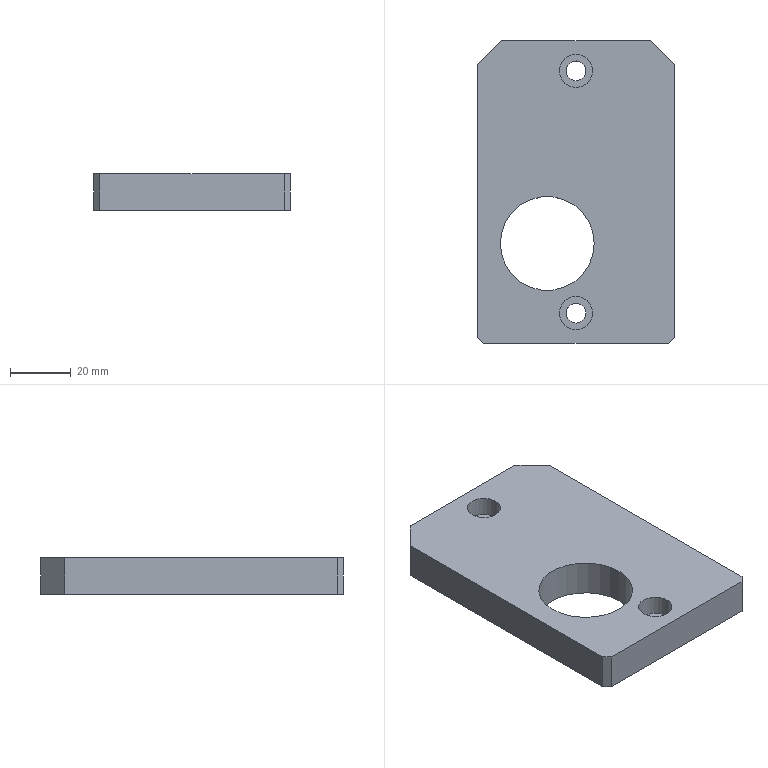Part | STEP file | P011002NM05-000 | 1 solid | 17 faces | box 65 x 100 x 12 mm | volume 66526 mm3 | plane 12 | cylinder 5 | commonest cylinder face diameters 6.5 x2 11 x2 31 x1
STEP:
#1=CARTESIAN_POINT('',(0.,0.,0.));
#2=DIRECTION('',(0.,0.,1.));
#3=DIRECTION('',(1.,0.,0.));
#4=AXIS2_PLACEMENT_3D('',#1,#2,#3);
#5=CARTESIAN_POINT('',(178.,-325.,9.));
#6=VERTEX_POINT('',#5);
#7=CARTESIAN_POINT('',(117.,-325.,9.));
#8=VERTEX_POINT('',#7);
#9=CARTESIAN_POINT('',(-325.,-325.,9.));
#10=DIRECTION('',(-1.,0.,0.));
#11=VECTOR('',#10,1.);
#12=LINE('',#9,#11);
#13=CARTESIAN_POINT('',(-325.,-325.,260.));
#14=DIRECTION('',(0.,1.,0.));
#15=DIRECTION('',(0.,0.,1.));
#16=AXIS2_PLACEMENT_3D('',#13,#14,#15);
#17=PLANE('',#16);
#18=CARTESIAN_POINT('',(-251.,0.));
#19=DIRECTION('',(0.,-1.));
#20=VECTOR('',#19,1.);
#21=LINE('',#18,#20);
#22=(GEOMETRIC_REPRESENTATION_CONTEXT(2)PARAMETRIC_REPRESENTATION_CONTEXT()REPRESENTATION_CONTEXT('',''));
#23=DEFINITIONAL_REPRESENTATION('',(#21),#22);
#24=PCURVE('',#17,#23);
#25=CARTESIAN_POINT('',(178.,-325.,9.));
#26=DIRECTION('',(0.,0.,1.));
#27=DIRECTION('',(1.,0.,0.));
#28=AXIS2_PLACEMENT_3D('',#25,#26,#27);
#29=PLANE('',#28);
#30=CARTESIAN_POINT('',(-503.,0.));
#31=DIRECTION('',(-1.,0.));
#32=VECTOR('',#31,1.);
#33=LINE('',#30,#32);
#34=(GEOMETRIC_REPRESENTATION_CONTEXT(2)PARAMETRIC_REPRESENTATION_CONTEXT()REPRESENTATION_CONTEXT('',''));
#35=DEFINITIONAL_REPRESENTATION('',(#33),#34);
#36=PCURVE('',#29,#35);
#37=SURFACE_CURVE('',#12,(#24,#36),.PCURVE_S1.);
#38=EDGE_CURVE('',#6,#8,#37,.T.);
#39=ORIENTED_EDGE('',*,*,#38,.F.);
#40=CARTESIAN_POINT('',(178.,-325.,21.));
#41=VERTEX_POINT('',#40);
#42=CARTESIAN_POINT('',(178.,-325.,260.));
#43=DIRECTION('',(0.,0.,1.));
#44=VECTOR('',#43,1.);
#45=LINE('',#42,#44);
#46=CARTESIAN_POINT('',(0.,503.));
#47=DIRECTION('',(1.,0.));
#48=VECTOR('',#47,1.);
#49=LINE('',#46,#48);
#50=(GEOMETRIC_REPRESENTATION_CONTEXT(2)PARAMETRIC_REPRESENTATION_CONTEXT()REPRESENTATION_CONTEXT('',''));
#51=DEFINITIONAL_REPRESENTATION('',(#49),#50);
#52=PCURVE('',#17,#51);
#53=CARTESIAN_POINT('',(180.,-323.,21.));
#54=DIRECTION('',(-0.7071,0.7071,0.));
#55=DIRECTION('',(-0.7071,-0.7071,0.));
#56=AXIS2_PLACEMENT_3D('',#53,#54,#55);
#57=PLANE('',#56);
#58=CARTESIAN_POINT('',(2.828,239.));
#59=DIRECTION('',(0.,1.));
#60=VECTOR('',#59,1.);
#61=LINE('',#58,#60);
#62=(GEOMETRIC_REPRESENTATION_CONTEXT(2)PARAMETRIC_REPRESENTATION_CONTEXT()REPRESENTATION_CONTEXT('',''));
#63=DEFINITIONAL_REPRESENTATION('',(#61),#62);
#64=PCURVE('',#57,#63);
#65=SURFACE_CURVE('',#45,(#52,#64),.PCURVE_S1.);
#66=EDGE_CURVE('',#6,#41,#65,.T.);
#67=ORIENTED_EDGE('',*,*,#66,.T.);
#68=CARTESIAN_POINT('',(117.,-325.,21.));
#69=VERTEX_POINT('',#68);
#70=CARTESIAN_POINT('',(-325.,-325.,21.));
#71=DIRECTION('',(-1.,0.,0.));
#72=VECTOR('',#71,1.);
#73=LINE('',#70,#72);
#74=CARTESIAN_POINT('',(-239.,0.));
#75=DIRECTION('',(0.,-1.));
#76=VECTOR('',#75,1.);
#77=LINE('',#74,#76);
#78=(GEOMETRIC_REPRESENTATION_CONTEXT(2)PARAMETRIC_REPRESENTATION_CONTEXT()REPRESENTATION_CONTEXT('',''));
#79=DEFINITIONAL_REPRESENTATION('',(#77),#78);
#80=PCURVE('',#17,#79);
#81=CARTESIAN_POINT('',(150.,-240.,21.));
#82=DIRECTION('',(0.,0.,1.));
#83=DIRECTION('',(1.,0.,0.));
#84=AXIS2_PLACEMENT_3D('',#81,#82,#83);
#85=PLANE('',#84);
#86=CARTESIAN_POINT('',(-475.,-85.));
#87=DIRECTION('',(-1.,0.));
#88=VECTOR('',#87,1.);
#89=LINE('',#86,#88);
#90=(GEOMETRIC_REPRESENTATION_CONTEXT(2)PARAMETRIC_REPRESENTATION_CONTEXT()REPRESENTATION_CONTEXT('',''));
#91=DEFINITIONAL_REPRESENTATION('',(#89),#90);
#92=PCURVE('',#85,#91);
#93=SURFACE_CURVE('',#73,(#80,#92),.PCURVE_S1.);
#94=EDGE_CURVE('',#41,#69,#93,.T.);
#95=ORIENTED_EDGE('',*,*,#94,.T.);
#96=CARTESIAN_POINT('',(117.,-325.,260.));
#97=DIRECTION('',(0.,0.,-1.));
#98=VECTOR('',#97,1.);
#99=LINE('',#96,#98);
#100=CARTESIAN_POINT('',(0.,442.));
#101=DIRECTION('',(-1.,0.));
#102=VECTOR('',#101,1.);
#103=LINE('',#100,#102);
#104=(GEOMETRIC_REPRESENTATION_CONTEXT(2)PARAMETRIC_REPRESENTATION_CONTEXT()REPRESENTATION_CONTEXT('',''));
#105=DEFINITIONAL_REPRESENTATION('',(#103),#104);
#106=PCURVE('',#17,#105);
#107=CARTESIAN_POINT('',(117.,-325.,260.));
#108=DIRECTION('',(0.7071,0.7071,0.));
#109=DIRECTION('',(-0.7071,0.7071,0.));
#110=AXIS2_PLACEMENT_3D('',#107,#108,#109);
#111=PLANE('',#110);
#112=CARTESIAN_POINT('',(0.,0.));
#113=DIRECTION('',(0.,-1.));
#114=VECTOR('',#113,1.);
#115=LINE('',#112,#114);
#116=(GEOMETRIC_REPRESENTATION_CONTEXT(2)PARAMETRIC_REPRESENTATION_CONTEXT()REPRESENTATION_CONTEXT('',''));
#117=DEFINITIONAL_REPRESENTATION('',(#115),#116);
#118=PCURVE('',#111,#117);
#119=SURFACE_CURVE('',#99,(#106,#118),.PCURVE_S1.);
#120=EDGE_CURVE('',#69,#8,#119,.T.);
#121=ORIENTED_EDGE('',*,*,#120,.T.);
#122=EDGE_LOOP('',(#39,#67,#95,#121));
#123=FACE_BOUND('',#122,.T.);
#124=ADVANCED_FACE('',(#123),#17,.F.);
#125=CARTESIAN_POINT('',(180.,-233.,9.));
#126=VERTEX_POINT('',#125);
#127=CARTESIAN_POINT('',(180.,-323.,9.));
#128=VERTEX_POINT('',#127);
#129=CARTESIAN_POINT('',(180.,-225.,9.));
#130=DIRECTION('',(0.,-1.,0.));
#131=VECTOR('',#130,1.);
#132=LINE('',#129,#131);
#133=CARTESIAN_POINT('',(180.,-225.,21.));
#134=DIRECTION('',(-1.,0.,0.));
#135=DIRECTION('',(0.,0.,-1.));
#136=AXIS2_PLACEMENT_3D('',#133,#134,#135);
#137=PLANE('',#136);
#138=CARTESIAN_POINT('',(12.,0.));
#139=DIRECTION('',(0.,1.));
#140=VECTOR('',#139,1.);
#141=LINE('',#138,#140);
#142=(GEOMETRIC_REPRESENTATION_CONTEXT(2)PARAMETRIC_REPRESENTATION_CONTEXT()REPRESENTATION_CONTEXT('',''));
#143=DEFINITIONAL_REPRESENTATION('',(#141),#142);
#144=PCURVE('',#137,#143);
#145=CARTESIAN_POINT('',(2.,100.));
#146=DIRECTION('',(0.,-1.));
#147=VECTOR('',#146,1.);
#148=LINE('',#145,#147);
#149=(GEOMETRIC_REPRESENTATION_CONTEXT(2)PARAMETRIC_REPRESENTATION_CONTEXT()REPRESENTATION_CONTEXT('',''));
#150=DEFINITIONAL_REPRESENTATION('',(#148),#149);
#151=PCURVE('',#29,#150);
#152=SURFACE_CURVE('',#132,(#144,#151),.PCURVE_S1.);
#153=EDGE_CURVE('',#126,#128,#152,.T.);
#154=ORIENTED_EDGE('',*,*,#153,.F.);
#155=CARTESIAN_POINT('',(180.,-233.,21.));
#156=VERTEX_POINT('',#155);
#157=CARTESIAN_POINT('',(180.,-233.,21.));
#158=DIRECTION('',(0.,0.,1.));
#159=VECTOR('',#158,1.);
#160=LINE('',#157,#159);
#161=CARTESIAN_POINT('',(0.,8.));
#162=DIRECTION('',(-1.,0.));
#163=VECTOR('',#162,1.);
#164=LINE('',#161,#163);
#165=(GEOMETRIC_REPRESENTATION_CONTEXT(2)PARAMETRIC_REPRESENTATION_CONTEXT()REPRESENTATION_CONTEXT('',''));
#166=DEFINITIONAL_REPRESENTATION('',(#164),#165);
#167=PCURVE('',#137,#166);
#168=CARTESIAN_POINT('',(172.,-225.,21.));
#169=DIRECTION('',(-0.7071,-0.7071,0.));
#170=DIRECTION('',(0.7071,-0.7071,0.));
#171=AXIS2_PLACEMENT_3D('',#168,#169,#170);
#172=PLANE('',#171);
#173=CARTESIAN_POINT('',(11.314,0.));
#174=DIRECTION('',(0.,1.));
#175=VECTOR('',#174,1.);
#176=LINE('',#173,#175);
#177=(GEOMETRIC_REPRESENTATION_CONTEXT(2)PARAMETRIC_REPRESENTATION_CONTEXT()REPRESENTATION_CONTEXT('',''));
#178=DEFINITIONAL_REPRESENTATION('',(#176),#177);
#179=PCURVE('',#172,#178);
#180=SURFACE_CURVE('',#160,(#167,#179),.PCURVE_S1.);
#181=EDGE_CURVE('',#126,#156,#180,.T.);
#182=ORIENTED_EDGE('',*,*,#181,.T.);
#183=CARTESIAN_POINT('',(180.,-323.,21.));
#184=VERTEX_POINT('',#183);
#185=CARTESIAN_POINT('',(180.,-225.,21.));
#186=DIRECTION('',(0.,-1.,0.));
#187=VECTOR('',#186,1.);
#188=LINE('',#185,#187);
#189=CARTESIAN_POINT('',(0.,0.));
#190=DIRECTION('',(0.,1.));
#191=VECTOR('',#190,1.);
#192=LINE('',#189,#191);
#193=(GEOMETRIC_REPRESENTATION_CONTEXT(2)PARAMETRIC_REPRESENTATION_CONTEXT()REPRESENTATION_CONTEXT('',''));
#194=DEFINITIONAL_REPRESENTATION('',(#192),#193);
#195=PCURVE('',#137,#194);
#196=CARTESIAN_POINT('',(30.,15.));
#197=DIRECTION('',(0.,-1.));
#198=VECTOR('',#197,1.);
#199=LINE('',#196,#198);
#200=(GEOMETRIC_REPRESENTATION_CONTEXT(2)PARAMETRIC_REPRESENTATION_CONTEXT()REPRESENTATION_CONTEXT('',''));
#201=DEFINITIONAL_REPRESENTATION('',(#199),#200);
#202=PCURVE('',#85,#201);
#203=SURFACE_CURVE('',#188,(#195,#202),.PCURVE_S1.);
#204=EDGE_CURVE('',#156,#184,#203,.T.);
#205=ORIENTED_EDGE('',*,*,#204,.T.);
#206=CARTESIAN_POINT('',(180.,-323.,21.));
#207=DIRECTION('',(0.,0.,-1.));
#208=VECTOR('',#207,1.);
#209=LINE('',#206,#208);
#210=CARTESIAN_POINT('',(0.,98.));
#211=DIRECTION('',(1.,0.));
#212=VECTOR('',#211,1.);
#213=LINE('',#210,#212);
#214=(GEOMETRIC_REPRESENTATION_CONTEXT(2)PARAMETRIC_REPRESENTATION_CONTEXT()REPRESENTATION_CONTEXT('',''));
#215=DEFINITIONAL_REPRESENTATION('',(#213),#214);
#216=PCURVE('',#137,#215);
#217=CARTESIAN_POINT('',(0.,0.));
#218=DIRECTION('',(0.,-1.));
#219=VECTOR('',#218,1.);
#220=LINE('',#217,#219);
#221=(GEOMETRIC_REPRESENTATION_CONTEXT(2)PARAMETRIC_REPRESENTATION_CONTEXT()REPRESENTATION_CONTEXT('',''));
#222=DEFINITIONAL_REPRESENTATION('',(#220),#221);
#223=PCURVE('',#57,#222);
#224=SURFACE_CURVE('',#209,(#216,#223),.PCURVE_S1.);
#225=EDGE_CURVE('',#184,#128,#224,.T.);
#226=ORIENTED_EDGE('',*,*,#225,.T.);
#227=EDGE_LOOP('',(#154,#182,#205,#226));
#228=FACE_BOUND('',#227,.T.);
#229=ADVANCED_FACE('',(#228),#137,.F.);
#230=CARTESIAN_POINT('',(123.,-225.,9.));
#231=VERTEX_POINT('',#230);
#232=CARTESIAN_POINT('',(172.,-225.,9.));
#233=VERTEX_POINT('',#232);
#234=CARTESIAN_POINT('',(125.,-225.,9.));
#235=DIRECTION('',(1.,0.,0.));
#236=VECTOR('',#235,1.);
#237=LINE('',#234,#236);
#238=CARTESIAN_POINT('',(125.,-225.,21.));
#239=DIRECTION('',(0.,-1.,0.));
#240=DIRECTION('',(0.,0.,-1.));
#241=AXIS2_PLACEMENT_3D('',#238,#239,#240);
#242=PLANE('',#241);
#243=CARTESIAN_POINT('',(12.,0.));
#244=DIRECTION('',(0.,1.));
#245=VECTOR('',#244,1.);
#246=LINE('',#243,#245);
#247=(GEOMETRIC_REPRESENTATION_CONTEXT(2)PARAMETRIC_REPRESENTATION_CONTEXT()REPRESENTATION_CONTEXT('',''));
#248=DEFINITIONAL_REPRESENTATION('',(#246),#247);
#249=PCURVE('',#242,#248);
#250=CARTESIAN_POINT('',(-53.,100.));
#251=DIRECTION('',(1.,0.));
#252=VECTOR('',#251,1.);
#253=LINE('',#250,#252);
#254=(GEOMETRIC_REPRESENTATION_CONTEXT(2)PARAMETRIC_REPRESENTATION_CONTEXT()REPRESENTATION_CONTEXT('',''));
#255=DEFINITIONAL_REPRESENTATION('',(#253),#254);
#256=PCURVE('',#29,#255);
#257=SURFACE_CURVE('',#237,(#249,#256),.PCURVE_S1.);
#258=EDGE_CURVE('',#231,#233,#257,.T.);
#259=ORIENTED_EDGE('',*,*,#258,.F.);
#260=CARTESIAN_POINT('',(123.,-225.,21.));
#261=VERTEX_POINT('',#260);
#262=CARTESIAN_POINT('',(123.,-225.,21.));
#263=DIRECTION('',(0.,0.,1.));
#264=VECTOR('',#263,1.);
#265=LINE('',#262,#264);
#266=CARTESIAN_POINT('',(0.,-2.));
#267=DIRECTION('',(-1.,0.));
#268=VECTOR('',#267,1.);
#269=LINE('',#266,#268);
#270=(GEOMETRIC_REPRESENTATION_CONTEXT(2)PARAMETRIC_REPRESENTATION_CONTEXT()REPRESENTATION_CONTEXT('',''));
#271=DEFINITIONAL_REPRESENTATION('',(#269),#270);
#272=PCURVE('',#242,#271);
#273=CARTESIAN_POINT('',(115.,-233.,21.));
#274=DIRECTION('',(0.7071,-0.7071,0.));
#275=DIRECTION('',(0.7071,0.7071,0.));
#276=AXIS2_PLACEMENT_3D('',#273,#274,#275);
#277=PLANE('',#276);
#278=CARTESIAN_POINT('',(11.314,0.));
#279=DIRECTION('',(0.,1.));
#280=VECTOR('',#279,1.);
#281=LINE('',#278,#280);
#282=(GEOMETRIC_REPRESENTATION_CONTEXT(2)PARAMETRIC_REPRESENTATION_CONTEXT()REPRESENTATION_CONTEXT('',''));
#283=DEFINITIONAL_REPRESENTATION('',(#281),#282);
#284=PCURVE('',#277,#283);
#285=SURFACE_CURVE('',#265,(#272,#284),.PCURVE_S1.);
#286=EDGE_CURVE('',#231,#261,#285,.T.);
#287=ORIENTED_EDGE('',*,*,#286,.T.);
#288=CARTESIAN_POINT('',(172.,-225.,21.));
#289=VERTEX_POINT('',#288);
#290=CARTESIAN_POINT('',(125.,-225.,21.));
#291=DIRECTION('',(1.,0.,0.));
#292=VECTOR('',#291,1.);
#293=LINE('',#290,#292);
#294=CARTESIAN_POINT('',(0.,0.));
#295=DIRECTION('',(0.,1.));
#296=VECTOR('',#295,1.);
#297=LINE('',#294,#296);
#298=(GEOMETRIC_REPRESENTATION_CONTEXT(2)PARAMETRIC_REPRESENTATION_CONTEXT()REPRESENTATION_CONTEXT('',''));
#299=DEFINITIONAL_REPRESENTATION('',(#297),#298);
#300=PCURVE('',#242,#299);
#301=CARTESIAN_POINT('',(-25.,15.));
#302=DIRECTION('',(1.,0.));
#303=VECTOR('',#302,1.);
#304=LINE('',#301,#303);
#305=(GEOMETRIC_REPRESENTATION_CONTEXT(2)PARAMETRIC_REPRESENTATION_CONTEXT()REPRESENTATION_CONTEXT('',''));
#306=DEFINITIONAL_REPRESENTATION('',(#304),#305);
#307=PCURVE('',#85,#306);
#308=SURFACE_CURVE('',#293,(#300,#307),.PCURVE_S1.);
#309=EDGE_CURVE('',#261,#289,#308,.T.);
#310=ORIENTED_EDGE('',*,*,#309,.T.);
#311=CARTESIAN_POINT('',(172.,-225.,21.));
#312=DIRECTION('',(0.,0.,-1.));
#313=VECTOR('',#312,1.);
#314=LINE('',#311,#313);
#315=CARTESIAN_POINT('',(0.,47.));
#316=DIRECTION('',(1.,0.));
#317=VECTOR('',#316,1.);
#318=LINE('',#315,#317);
#319=(GEOMETRIC_REPRESENTATION_CONTEXT(2)PARAMETRIC_REPRESENTATION_CONTEXT()REPRESENTATION_CONTEXT('',''));
#320=DEFINITIONAL_REPRESENTATION('',(#318),#319);
#321=PCURVE('',#242,#320);
#322=CARTESIAN_POINT('',(0.,0.));
#323=DIRECTION('',(0.,-1.));
#324=VECTOR('',#323,1.);
#325=LINE('',#322,#324);
#326=(GEOMETRIC_REPRESENTATION_CONTEXT(2)PARAMETRIC_REPRESENTATION_CONTEXT()REPRESENTATION_CONTEXT('',''));
#327=DEFINITIONAL_REPRESENTATION('',(#325),#326);
#328=PCURVE('',#172,#327);
#329=SURFACE_CURVE('',#314,(#321,#328),.PCURVE_S1.);
#330=EDGE_CURVE('',#289,#233,#329,.T.);
#331=ORIENTED_EDGE('',*,*,#330,.T.);
#332=EDGE_LOOP('',(#259,#287,#310,#331));
#333=FACE_BOUND('',#332,.T.);
#334=ADVANCED_FACE('',(#333),#242,.F.);
#335=CARTESIAN_POINT('',(147.5,-240.5,21.));
#336=VERTEX_POINT('',#335);
#337=CARTESIAN_POINT('',(147.5,-235.,21.));
#338=DIRECTION('',(0.,0.,1.));
#339=DIRECTION('',(0.,-1.,0.));
#340=AXIS2_PLACEMENT_3D('',#337,#338,#339);
#341=CIRCLE('',#340,5.5);
#342=CARTESIAN_POINT('',(-2.5,5.));
#343=DIRECTION('',(0.,-1.));
#344=AXIS2_PLACEMENT_2D('',#342,#343);
#345=CIRCLE('',#344,5.5);
#346=(GEOMETRIC_REPRESENTATION_CONTEXT(2)PARAMETRIC_REPRESENTATION_CONTEXT()REPRESENTATION_CONTEXT('',''));
#347=DEFINITIONAL_REPRESENTATION('',(#345),#346);
#348=PCURVE('',#85,#347);
#349=CARTESIAN_POINT('',(147.5,-235.,22.));
#350=DIRECTION('',(0.,0.,1.));
#351=DIRECTION('',(0.,-1.,0.));
#352=AXIS2_PLACEMENT_3D('',#349,#350,#351);
#353=CYLINDRICAL_SURFACE('',#352,5.5);
#354=CARTESIAN_POINT('',(0.,-1.));
#355=DIRECTION('',(1.,0.));
#356=VECTOR('',#355,1.);
#357=LINE('',#354,#356);
#358=(GEOMETRIC_REPRESENTATION_CONTEXT(2)PARAMETRIC_REPRESENTATION_CONTEXT()REPRESENTATION_CONTEXT('',''));
#359=DEFINITIONAL_REPRESENTATION('',(#357),#358);
#360=PCURVE('',#353,#359);
#361=SURFACE_CURVE('',#341,(#348,#360),.PCURVE_S1.);
#362=EDGE_CURVE('',#336,#336,#361,.T.);
#363=ORIENTED_EDGE('',*,*,#362,.F.);
#364=EDGE_LOOP('',(#363));
#365=FACE_BOUND('',#364,.T.);
#366=CARTESIAN_POINT('',(147.5,-320.5,21.));
#367=VERTEX_POINT('',#366);
#368=CARTESIAN_POINT('',(147.5,-315.,21.));
#369=DIRECTION('',(0.,0.,1.));
#370=DIRECTION('',(0.,-1.,0.));
#371=AXIS2_PLACEMENT_3D('',#368,#369,#370);
#372=CIRCLE('',#371,5.5);
#373=CARTESIAN_POINT('',(-2.5,-75.));
#374=DIRECTION('',(0.,-1.));
#375=AXIS2_PLACEMENT_2D('',#373,#374);
#376=CIRCLE('',#375,5.5);
#377=(GEOMETRIC_REPRESENTATION_CONTEXT(2)PARAMETRIC_REPRESENTATION_CONTEXT()REPRESENTATION_CONTEXT('',''));
#378=DEFINITIONAL_REPRESENTATION('',(#376),#377);
#379=PCURVE('',#85,#378);
#380=CARTESIAN_POINT('',(147.5,-315.,22.));
#381=DIRECTION('',(0.,0.,1.));
#382=DIRECTION('',(0.,-1.,0.));
#383=AXIS2_PLACEMENT_3D('',#380,#381,#382);
#384=CYLINDRICAL_SURFACE('',#383,5.5);
#385=CARTESIAN_POINT('',(0.,-1.));
#386=DIRECTION('',(1.,0.));
#387=VECTOR('',#386,1.);
#388=LINE('',#385,#387);
#389=(GEOMETRIC_REPRESENTATION_CONTEXT(2)PARAMETRIC_REPRESENTATION_CONTEXT()REPRESENTATION_CONTEXT('',''));
#390=DEFINITIONAL_REPRESENTATION('',(#388),#389);
#391=PCURVE('',#384,#390);
#392=SURFACE_CURVE('',#372,(#379,#391),.PCURVE_S1.);
#393=EDGE_CURVE('',#367,#367,#392,.T.);
#394=ORIENTED_EDGE('',*,*,#393,.F.);
#395=EDGE_LOOP('',(#394));
#396=FACE_BOUND('',#395,.T.);
#397=CARTESIAN_POINT('',(153.5,-292.,21.));
#398=VERTEX_POINT('',#397);
#399=CARTESIAN_POINT('',(138.,-292.,21.));
#400=DIRECTION('',(0.,0.,1.));
#401=DIRECTION('',(1.,0.,0.));
#402=AXIS2_PLACEMENT_3D('',#399,#400,#401);
#403=CIRCLE('',#402,15.5);
#404=CARTESIAN_POINT('',(-12.,-52.));
#405=DIRECTION('',(1.,0.));
#406=AXIS2_PLACEMENT_2D('',#404,#405);
#407=CIRCLE('',#406,15.5);
#408=(GEOMETRIC_REPRESENTATION_CONTEXT(2)PARAMETRIC_REPRESENTATION_CONTEXT()REPRESENTATION_CONTEXT('',''));
#409=DEFINITIONAL_REPRESENTATION('',(#407),#408);
#410=PCURVE('',#85,#409);
#411=CARTESIAN_POINT('',(138.,-292.,539.));
#412=DIRECTION('',(0.,0.,-1.));
#413=DIRECTION('',(1.,0.,0.));
#414=AXIS2_PLACEMENT_3D('',#411,#412,#413);
#415=CYLINDRICAL_SURFACE('',#414,15.5);
#416=CARTESIAN_POINT('',(6.283,518.));
#417=DIRECTION('',(-1.,0.));
#418=VECTOR('',#417,1.);
#419=LINE('',#416,#418);
#420=(GEOMETRIC_REPRESENTATION_CONTEXT(2)PARAMETRIC_REPRESENTATION_CONTEXT()REPRESENTATION_CONTEXT('',''));
#421=DEFINITIONAL_REPRESENTATION('',(#419),#420);
#422=PCURVE('',#415,#421);
#423=SURFACE_CURVE('',#403,(#410,#422),.PCURVE_S1.);
#424=EDGE_CURVE('',#398,#398,#423,.T.);
#425=ORIENTED_EDGE('',*,*,#424,.F.);
#426=EDGE_LOOP('',(#425));
#427=FACE_BOUND('',#426,.T.);
#428=ORIENTED_EDGE('',*,*,#94,.F.);
#429=CARTESIAN_POINT('',(206.5,-296.5,21.));
#430=DIRECTION('',(0.7071,0.7071,0.));
#431=VECTOR('',#430,1.);
#432=LINE('',#429,#431);
#433=CARTESIAN_POINT('',(56.5,-56.5));
#434=DIRECTION('',(0.7071,0.7071));
#435=VECTOR('',#434,1.);
#436=LINE('',#433,#435);
#437=(GEOMETRIC_REPRESENTATION_CONTEXT(2)PARAMETRIC_REPRESENTATION_CONTEXT()REPRESENTATION_CONTEXT('',''));
#438=DEFINITIONAL_REPRESENTATION('',(#436),#437);
#439=PCURVE('',#85,#438);
#440=CARTESIAN_POINT('',(-37.477,0.));
#441=DIRECTION('',(-1.,0.));
#442=VECTOR('',#441,1.);
#443=LINE('',#440,#442);
#444=(GEOMETRIC_REPRESENTATION_CONTEXT(2)PARAMETRIC_REPRESENTATION_CONTEXT()REPRESENTATION_CONTEXT('',''));
#445=DEFINITIONAL_REPRESENTATION('',(#443),#444);
#446=PCURVE('',#57,#445);
#447=SURFACE_CURVE('',#432,(#439,#446),.PCURVE_S1.);
#448=EDGE_CURVE('',#41,#184,#447,.T.);
#449=ORIENTED_EDGE('',*,*,#448,.T.);
#450=ORIENTED_EDGE('',*,*,#204,.F.);
#451=CARTESIAN_POINT('',(168.5,-221.5,21.));
#452=DIRECTION('',(-0.7071,0.7071,0.));
#453=VECTOR('',#452,1.);
#454=LINE('',#451,#453);
#455=CARTESIAN_POINT('',(18.5,18.5));
#456=DIRECTION('',(-0.7071,0.7071));
#457=VECTOR('',#456,1.);
#458=LINE('',#455,#457);
#459=(GEOMETRIC_REPRESENTATION_CONTEXT(2)PARAMETRIC_REPRESENTATION_CONTEXT()REPRESENTATION_CONTEXT('',''));
#460=DEFINITIONAL_REPRESENTATION('',(#458),#459);
#461=PCURVE('',#85,#460);
#462=CARTESIAN_POINT('',(-4.95,0.));
#463=DIRECTION('',(-1.,0.));
#464=VECTOR('',#463,1.);
#465=LINE('',#462,#464);
#466=(GEOMETRIC_REPRESENTATION_CONTEXT(2)PARAMETRIC_REPRESENTATION_CONTEXT()REPRESENTATION_CONTEXT('',''));
#467=DEFINITIONAL_REPRESENTATION('',(#465),#466);
#468=PCURVE('',#172,#467);
#469=SURFACE_CURVE('',#454,(#461,#468),.PCURVE_S1.);
#470=EDGE_CURVE('',#156,#289,#469,.T.);
#471=ORIENTED_EDGE('',*,*,#470,.T.);
#472=ORIENTED_EDGE('',*,*,#309,.F.);
#473=CARTESIAN_POINT('',(115.,-233.,21.));
#474=VERTEX_POINT('',#473);
#475=CARTESIAN_POINT('',(129.,-219.,21.));
#476=DIRECTION('',(-0.7071,-0.7071,0.));
#477=VECTOR('',#476,1.);
#478=LINE('',#475,#477);
#479=CARTESIAN_POINT('',(-21.,21.));
#480=DIRECTION('',(-0.7071,-0.7071));
#481=VECTOR('',#480,1.);
#482=LINE('',#479,#481);
#483=(GEOMETRIC_REPRESENTATION_CONTEXT(2)PARAMETRIC_REPRESENTATION_CONTEXT()REPRESENTATION_CONTEXT('',''));
#484=DEFINITIONAL_REPRESENTATION('',(#482),#483);
#485=PCURVE('',#85,#484);
#486=CARTESIAN_POINT('',(19.799,0.));
#487=DIRECTION('',(-1.,0.));
#488=VECTOR('',#487,1.);
#489=LINE('',#486,#488);
#490=(GEOMETRIC_REPRESENTATION_CONTEXT(2)PARAMETRIC_REPRESENTATION_CONTEXT()REPRESENTATION_CONTEXT('',''));
#491=DEFINITIONAL_REPRESENTATION('',(#489),#490);
#492=PCURVE('',#277,#491);
#493=SURFACE_CURVE('',#478,(#485,#492),.PCURVE_S1.);
#494=EDGE_CURVE('',#261,#474,#493,.T.);
#495=ORIENTED_EDGE('',*,*,#494,.T.);
#496=CARTESIAN_POINT('',(115.,-323.,21.));
#497=VERTEX_POINT('',#496);
#498=CARTESIAN_POINT('',(115.,-255.,21.));
#499=DIRECTION('',(0.,1.,0.));
#500=VECTOR('',#499,1.);
#501=LINE('',#498,#500);
#502=CARTESIAN_POINT('',(-35.,-15.));
#503=DIRECTION('',(0.,1.));
#504=VECTOR('',#503,1.);
#505=LINE('',#502,#504);
#506=(GEOMETRIC_REPRESENTATION_CONTEXT(2)PARAMETRIC_REPRESENTATION_CONTEXT()REPRESENTATION_CONTEXT('',''));
#507=DEFINITIONAL_REPRESENTATION('',(#505),#506);
#508=PCURVE('',#85,#507);
#509=CARTESIAN_POINT('',(115.,-255.,21.));
#510=DIRECTION('',(1.,0.,0.));
#511=DIRECTION('',(0.,0.,1.));
#512=AXIS2_PLACEMENT_3D('',#509,#510,#511);
#513=PLANE('',#512);
#514=CARTESIAN_POINT('',(0.,0.));
#515=DIRECTION('',(0.,-1.));
#516=VECTOR('',#515,1.);
#517=LINE('',#514,#516);
#518=(GEOMETRIC_REPRESENTATION_CONTEXT(2)PARAMETRIC_REPRESENTATION_CONTEXT()REPRESENTATION_CONTEXT('',''));
#519=DEFINITIONAL_REPRESENTATION('',(#517),#518);
#520=PCURVE('',#513,#519);
#521=SURFACE_CURVE('',#501,(#508,#520),.PCURVE_S1.);
#522=EDGE_CURVE('',#497,#474,#521,.T.);
#523=ORIENTED_EDGE('',*,*,#522,.F.);
#524=CARTESIAN_POINT('',(91.,-299.,21.));
#525=DIRECTION('',(0.7071,-0.7071,0.));
#526=VECTOR('',#525,1.);
#527=LINE('',#524,#526);
#528=CARTESIAN_POINT('',(-59.,-59.));
#529=DIRECTION('',(0.7071,-0.7071));
#530=VECTOR('',#529,1.);
#531=LINE('',#528,#530);
#532=(GEOMETRIC_REPRESENTATION_CONTEXT(2)PARAMETRIC_REPRESENTATION_CONTEXT()REPRESENTATION_CONTEXT('',''));
#533=DEFINITIONAL_REPRESENTATION('',(#531),#532);
#534=PCURVE('',#85,#533);
#535=CARTESIAN_POINT('',(36.77,-239.));
#536=DIRECTION('',(-1.,0.));
#537=VECTOR('',#536,1.);
#538=LINE('',#535,#537);
#539=(GEOMETRIC_REPRESENTATION_CONTEXT(2)PARAMETRIC_REPRESENTATION_CONTEXT()REPRESENTATION_CONTEXT('',''));
#540=DEFINITIONAL_REPRESENTATION('',(#538),#539);
#541=PCURVE('',#111,#540);
#542=SURFACE_CURVE('',#527,(#534,#541),.PCURVE_S1.);
#543=EDGE_CURVE('',#497,#69,#542,.T.);
#544=ORIENTED_EDGE('',*,*,#543,.T.);
#545=EDGE_LOOP('',(#428,#449,#450,#471,#472,#495,#523,#544));
#546=FACE_BOUND('',#545,.T.);
#547=ADVANCED_FACE('',(#365,#396,#427,#546),#85,.T.);
#548=CARTESIAN_POINT('',(115.,-323.,9.));
#549=VERTEX_POINT('',#548);
#550=CARTESIAN_POINT('',(115.,-233.,9.));
#551=VERTEX_POINT('',#550);
#552=CARTESIAN_POINT('',(115.,-255.,9.));
#553=DIRECTION('',(0.,1.,0.));
#554=VECTOR('',#553,1.);
#555=LINE('',#552,#554);
#556=CARTESIAN_POINT('',(-12.,0.));
#557=DIRECTION('',(0.,-1.));
#558=VECTOR('',#557,1.);
#559=LINE('',#556,#558);
#560=(GEOMETRIC_REPRESENTATION_CONTEXT(2)PARAMETRIC_REPRESENTATION_CONTEXT()REPRESENTATION_CONTEXT('',''));
#561=DEFINITIONAL_REPRESENTATION('',(#559),#560);
#562=PCURVE('',#513,#561);
#563=CARTESIAN_POINT('',(-63.,70.));
#564=DIRECTION('',(0.,1.));
#565=VECTOR('',#564,1.);
#566=LINE('',#563,#565);
#567=(GEOMETRIC_REPRESENTATION_CONTEXT(2)PARAMETRIC_REPRESENTATION_CONTEXT()REPRESENTATION_CONTEXT('',''));
#568=DEFINITIONAL_REPRESENTATION('',(#566),#567);
#569=PCURVE('',#29,#568);
#570=SURFACE_CURVE('',#555,(#562,#569),.PCURVE_S1.);
#571=EDGE_CURVE('',#549,#551,#570,.T.);
#572=ORIENTED_EDGE('',*,*,#571,.F.);
#573=CARTESIAN_POINT('',(115.,-323.,21.));
#574=DIRECTION('',(0.,0.,1.));
#575=VECTOR('',#574,1.);
#576=LINE('',#573,#575);
#577=CARTESIAN_POINT('',(0.,68.));
#578=DIRECTION('',(1.,0.));
#579=VECTOR('',#578,1.);
#580=LINE('',#577,#579);
#581=(GEOMETRIC_REPRESENTATION_CONTEXT(2)PARAMETRIC_REPRESENTATION_CONTEXT()REPRESENTATION_CONTEXT('',''));
#582=DEFINITIONAL_REPRESENTATION('',(#580),#581);
#583=PCURVE('',#513,#582);
#584=CARTESIAN_POINT('',(2.828,-239.));
#585=DIRECTION('',(0.,1.));
#586=VECTOR('',#585,1.);
#587=LINE('',#584,#586);
#588=(GEOMETRIC_REPRESENTATION_CONTEXT(2)PARAMETRIC_REPRESENTATION_CONTEXT()REPRESENTATION_CONTEXT('',''));
#589=DEFINITIONAL_REPRESENTATION('',(#587),#588);
#590=PCURVE('',#111,#589);
#591=SURFACE_CURVE('',#576,(#583,#590),.PCURVE_S1.);
#592=EDGE_CURVE('',#549,#497,#591,.T.);
#593=ORIENTED_EDGE('',*,*,#592,.T.);
#594=ORIENTED_EDGE('',*,*,#522,.T.);
#595=CARTESIAN_POINT('',(115.,-233.,21.));
#596=DIRECTION('',(0.,0.,-1.));
#597=VECTOR('',#596,1.);
#598=LINE('',#595,#597);
#599=CARTESIAN_POINT('',(0.,-22.));
#600=DIRECTION('',(-1.,0.));
#601=VECTOR('',#600,1.);
#602=LINE('',#599,#601);
#603=(GEOMETRIC_REPRESENTATION_CONTEXT(2)PARAMETRIC_REPRESENTATION_CONTEXT()REPRESENTATION_CONTEXT('',''));
#604=DEFINITIONAL_REPRESENTATION('',(#602),#603);
#605=PCURVE('',#513,#604);
#606=CARTESIAN_POINT('',(0.,0.));
#607=DIRECTION('',(0.,-1.));
#608=VECTOR('',#607,1.);
#609=LINE('',#606,#608);
#610=(GEOMETRIC_REPRESENTATION_CONTEXT(2)PARAMETRIC_REPRESENTATION_CONTEXT()REPRESENTATION_CONTEXT('',''));
#611=DEFINITIONAL_REPRESENTATION('',(#609),#610);
#612=PCURVE('',#277,#611);
#613=SURFACE_CURVE('',#598,(#605,#612),.PCURVE_S1.);
#614=EDGE_CURVE('',#474,#551,#613,.T.);
#615=ORIENTED_EDGE('',*,*,#614,.T.);
#616=EDGE_LOOP('',(#572,#593,#594,#615));
#617=FACE_BOUND('',#616,.T.);
#618=ADVANCED_FACE('',(#617),#513,.F.);
#619=CARTESIAN_POINT('',(172.,-225.,9.));
#620=DIRECTION('',(0.7071,-0.7071,0.));
#621=VECTOR('',#620,1.);
#622=LINE('',#619,#621);
#623=CARTESIAN_POINT('',(0.,-12.));
#624=DIRECTION('',(1.,0.));
#625=VECTOR('',#624,1.);
#626=LINE('',#623,#625);
#627=(GEOMETRIC_REPRESENTATION_CONTEXT(2)PARAMETRIC_REPRESENTATION_CONTEXT()REPRESENTATION_CONTEXT('',''));
#628=DEFINITIONAL_REPRESENTATION('',(#626),#627);
#629=PCURVE('',#172,#628);
#630=CARTESIAN_POINT('',(-6.,100.));
#631=DIRECTION('',(0.7071,-0.7071));
#632=VECTOR('',#631,1.);
#633=LINE('',#630,#632);
#634=(GEOMETRIC_REPRESENTATION_CONTEXT(2)PARAMETRIC_REPRESENTATION_CONTEXT()REPRESENTATION_CONTEXT('',''));
#635=DEFINITIONAL_REPRESENTATION('',(#633),#634);
#636=PCURVE('',#29,#635);
#637=SURFACE_CURVE('',#622,(#629,#636),.PCURVE_S1.);
#638=EDGE_CURVE('',#233,#126,#637,.T.);
#639=ORIENTED_EDGE('',*,*,#638,.F.);
#640=ORIENTED_EDGE('',*,*,#330,.F.);
#641=ORIENTED_EDGE('',*,*,#470,.F.);
#642=ORIENTED_EDGE('',*,*,#181,.F.);
#643=EDGE_LOOP('',(#639,#640,#641,#642));
#644=FACE_BOUND('',#643,.T.);
#645=ADVANCED_FACE('',(#644),#172,.F.);
#646=CARTESIAN_POINT('',(115.,-233.,9.));
#647=DIRECTION('',(0.7071,0.7071,0.));
#648=VECTOR('',#647,1.);
#649=LINE('',#646,#648);
#650=CARTESIAN_POINT('',(0.,-12.));
#651=DIRECTION('',(1.,0.));
#652=VECTOR('',#651,1.);
#653=LINE('',#650,#652);
#654=(GEOMETRIC_REPRESENTATION_CONTEXT(2)PARAMETRIC_REPRESENTATION_CONTEXT()REPRESENTATION_CONTEXT('',''));
#655=DEFINITIONAL_REPRESENTATION('',(#653),#654);
#656=PCURVE('',#277,#655);
#657=CARTESIAN_POINT('',(-63.,92.));
#658=DIRECTION('',(0.7071,0.7071));
#659=VECTOR('',#658,1.);
#660=LINE('',#657,#659);
#661=(GEOMETRIC_REPRESENTATION_CONTEXT(2)PARAMETRIC_REPRESENTATION_CONTEXT()REPRESENTATION_CONTEXT('',''));
#662=DEFINITIONAL_REPRESENTATION('',(#660),#661);
#663=PCURVE('',#29,#662);
#664=SURFACE_CURVE('',#649,(#656,#663),.PCURVE_S1.);
#665=EDGE_CURVE('',#551,#231,#664,.T.);
#666=ORIENTED_EDGE('',*,*,#665,.F.);
#667=ORIENTED_EDGE('',*,*,#614,.F.);
#668=ORIENTED_EDGE('',*,*,#494,.F.);
#669=ORIENTED_EDGE('',*,*,#286,.F.);
#670=EDGE_LOOP('',(#666,#667,#668,#669));
#671=FACE_BOUND('',#670,.T.);
#672=ADVANCED_FACE('',(#671),#277,.F.);
#673=CARTESIAN_POINT('',(180.,-323.,9.));
#674=DIRECTION('',(-0.7071,-0.7071,0.));
#675=VECTOR('',#674,1.);
#676=LINE('',#673,#675);
#677=CARTESIAN_POINT('',(0.,-12.));
#678=DIRECTION('',(1.,0.));
#679=VECTOR('',#678,1.);
#680=LINE('',#677,#679);
#681=(GEOMETRIC_REPRESENTATION_CONTEXT(2)PARAMETRIC_REPRESENTATION_CONTEXT()REPRESENTATION_CONTEXT('',''));
#682=DEFINITIONAL_REPRESENTATION('',(#680),#681);
#683=PCURVE('',#57,#682);
#684=CARTESIAN_POINT('',(2.,2.));
#685=DIRECTION('',(-0.7071,-0.7071));
#686=VECTOR('',#685,1.);
#687=LINE('',#684,#686);
#688=(GEOMETRIC_REPRESENTATION_CONTEXT(2)PARAMETRIC_REPRESENTATION_CONTEXT()REPRESENTATION_CONTEXT('',''));
#689=DEFINITIONAL_REPRESENTATION('',(#687),#688);
#690=PCURVE('',#29,#689);
#691=SURFACE_CURVE('',#676,(#683,#690),.PCURVE_S1.);
#692=EDGE_CURVE('',#128,#6,#691,.T.);
#693=ORIENTED_EDGE('',*,*,#692,.F.);
#694=ORIENTED_EDGE('',*,*,#225,.F.);
#695=ORIENTED_EDGE('',*,*,#448,.F.);
#696=ORIENTED_EDGE('',*,*,#66,.F.);
#697=EDGE_LOOP('',(#693,#694,#695,#696));
#698=FACE_BOUND('',#697,.T.);
#699=ADVANCED_FACE('',(#698),#57,.F.);
#700=CARTESIAN_POINT('',(117.,-325.,9.));
#701=DIRECTION('',(-0.7071,0.7071,0.));
#702=VECTOR('',#701,1.);
#703=LINE('',#700,#702);
#704=CARTESIAN_POINT('',(0.,-251.));
#705=DIRECTION('',(1.,0.));
#706=VECTOR('',#705,1.);
#707=LINE('',#704,#706);
#708=(GEOMETRIC_REPRESENTATION_CONTEXT(2)PARAMETRIC_REPRESENTATION_CONTEXT()REPRESENTATION_CONTEXT('',''));
#709=DEFINITIONAL_REPRESENTATION('',(#707),#708);
#710=PCURVE('',#111,#709);
#711=CARTESIAN_POINT('',(-61.,0.));
#712=DIRECTION('',(-0.7071,0.7071));
#713=VECTOR('',#712,1.);
#714=LINE('',#711,#713);
#715=(GEOMETRIC_REPRESENTATION_CONTEXT(2)PARAMETRIC_REPRESENTATION_CONTEXT()REPRESENTATION_CONTEXT('',''));
#716=DEFINITIONAL_REPRESENTATION('',(#714),#715);
#717=PCURVE('',#29,#716);
#718=SURFACE_CURVE('',#703,(#710,#717),.PCURVE_S1.);
#719=EDGE_CURVE('',#8,#549,#718,.T.);
#720=ORIENTED_EDGE('',*,*,#719,.F.);
#721=ORIENTED_EDGE('',*,*,#120,.F.);
#722=ORIENTED_EDGE('',*,*,#543,.F.);
#723=ORIENTED_EDGE('',*,*,#592,.F.);
#724=EDGE_LOOP('',(#720,#721,#722,#723));
#725=FACE_BOUND('',#724,.T.);
#726=ADVANCED_FACE('',(#725),#111,.F.);
#727=CARTESIAN_POINT('',(153.5,-292.,9.));
#728=VERTEX_POINT('',#727);
#729=CARTESIAN_POINT('',(138.,-292.,9.));
#730=DIRECTION('',(0.,0.,-1.));
#731=DIRECTION('',(1.,0.,0.));
#732=AXIS2_PLACEMENT_3D('',#729,#730,#731);
#733=CIRCLE('',#732,15.5);
#734=CARTESIAN_POINT('',(0.,530.));
#735=DIRECTION('',(1.,0.));
#736=VECTOR('',#735,1.);
#737=LINE('',#734,#736);
#738=(GEOMETRIC_REPRESENTATION_CONTEXT(2)PARAMETRIC_REPRESENTATION_CONTEXT()REPRESENTATION_CONTEXT('',''));
#739=DEFINITIONAL_REPRESENTATION('',(#737),#738);
#740=PCURVE('',#415,#739);
#741=CARTESIAN_POINT('',(-24.5,33.));
#742=CARTESIAN_POINT('',(-24.5,6.153));
#743=CARTESIAN_POINT('',(-47.75,19.577));
#744=CARTESIAN_POINT('',(-71.,33.));
#745=CARTESIAN_POINT('',(-47.75,46.423));
#746=CARTESIAN_POINT('',(-24.5,59.847));
#747=CARTESIAN_POINT('',(-24.5,33.));
#748=(BOUNDED_CURVE()B_SPLINE_CURVE(2,(#741,#742,#743,#744,#745,#746,#747),.UNSPECIFIED.,.T.,.F.)B_SPLINE_CURVE_WITH_KNOTS((1,2,2,2,2,1),(-2.094,0.,2.094,4.189,6.283,8.378),.UNSPECIFIED.)CURVE()GEOMETRIC_REPRESENTATION_ITEM()RATIONAL_B_SPLINE_CURVE((1.,0.5,1.,0.5,1.,0.5,1.))REPRESENTATION_ITEM(''));
#749=(GEOMETRIC_REPRESENTATION_CONTEXT(2)PARAMETRIC_REPRESENTATION_CONTEXT()REPRESENTATION_CONTEXT('',''));
#750=DEFINITIONAL_REPRESENTATION('',(#748),#749);
#751=PCURVE('',#29,#750);
#752=SURFACE_CURVE('',#733,(#740,#751),.PCURVE_S1.);
#753=EDGE_CURVE('',#728,#728,#752,.T.);
#754=ORIENTED_EDGE('',*,*,#753,.F.);
#755=CARTESIAN_POINT('',(153.5,-292.,21.));
#756=CARTESIAN_POINT('',(153.5,-292.,9.));
#757=B_SPLINE_CURVE_WITH_KNOTS('',1,(#755,#756),.UNSPECIFIED.,.F.,.F.,(2,2),(518.,530.),.PIECEWISE_BEZIER_KNOTS.);
#758=CARTESIAN_POINT('',(0.,0.));
#759=DIRECTION('',(0.,1.));
#760=VECTOR('',#759,1.);
#761=LINE('',#758,#760);
#762=(GEOMETRIC_REPRESENTATION_CONTEXT(2)PARAMETRIC_REPRESENTATION_CONTEXT()REPRESENTATION_CONTEXT('',''));
#763=DEFINITIONAL_REPRESENTATION('',(#761),#762);
#764=PCURVE('',#415,#763);
#765=CARTESIAN_POINT('',(6.283,0.));
#766=DIRECTION('',(0.,1.));
#767=VECTOR('',#766,1.);
#768=LINE('',#765,#767);
#769=(GEOMETRIC_REPRESENTATION_CONTEXT(2)PARAMETRIC_REPRESENTATION_CONTEXT()REPRESENTATION_CONTEXT('',''));
#770=DEFINITIONAL_REPRESENTATION('',(#768),#769);
#771=PCURVE('',#415,#770);
#772=SEAM_CURVE('',#757,(#764,#771),.PCURVE_S1.);
#773=EDGE_CURVE('',#398,#728,#772,.T.);
#774=ORIENTED_EDGE('',*,*,#773,.F.);
#775=ORIENTED_EDGE('',*,*,#424,.F.);
#776=ORIENTED_EDGE('',*,*,#773,.T.);
#777=EDGE_LOOP('',(#754,#774,#775,#776));
#778=FACE_BOUND('',#777,.F.);
#779=ADVANCED_FACE('',(#778),#415,.F.);
#780=CARTESIAN_POINT('',(147.5,-318.25,14.5));
#781=VERTEX_POINT('',#780);
#782=CARTESIAN_POINT('',(147.5,-315.,14.5));
#783=DIRECTION('',(0.,0.,1.));
#784=DIRECTION('',(0.,-1.,0.));
#785=AXIS2_PLACEMENT_3D('',#782,#783,#784);
#786=CIRCLE('',#785,3.25);
#787=CARTESIAN_POINT('',(147.5,-315.,22.));
#788=DIRECTION('',(0.,0.,1.));
#789=DIRECTION('',(0.,-1.,0.));
#790=AXIS2_PLACEMENT_3D('',#787,#788,#789);
#791=CYLINDRICAL_SURFACE('',#790,3.25);
#792=CARTESIAN_POINT('',(0.,-7.5));
#793=DIRECTION('',(1.,0.));
#794=VECTOR('',#793,1.);
#795=LINE('',#792,#794);
#796=(GEOMETRIC_REPRESENTATION_CONTEXT(2)PARAMETRIC_REPRESENTATION_CONTEXT()REPRESENTATION_CONTEXT('',''));
#797=DEFINITIONAL_REPRESENTATION('',(#795),#796);
#798=PCURVE('',#791,#797);
#799=CARTESIAN_POINT('',(147.5,-315.,14.5));
#800=DIRECTION('',(0.,0.,1.));
#801=DIRECTION('',(0.,-1.,0.));
#802=AXIS2_PLACEMENT_3D('',#799,#800,#801);
#803=PLANE('',#802);
#804=CARTESIAN_POINT('',(0.,0.));
#805=DIRECTION('',(1.,0.));
#806=AXIS2_PLACEMENT_2D('',#804,#805);
#807=CIRCLE('',#806,3.25);
#808=(GEOMETRIC_REPRESENTATION_CONTEXT(2)PARAMETRIC_REPRESENTATION_CONTEXT()REPRESENTATION_CONTEXT('',''));
#809=DEFINITIONAL_REPRESENTATION('',(#807),#808);
#810=PCURVE('',#803,#809);
#811=SURFACE_CURVE('',#786,(#798,#810),.PCURVE_S1.);
#812=EDGE_CURVE('',#781,#781,#811,.T.);
#813=ORIENTED_EDGE('',*,*,#812,.F.);
#814=CARTESIAN_POINT('',(147.5,-318.25,9.));
#815=VERTEX_POINT('',#814);
#816=CARTESIAN_POINT('',(147.5,-318.25,9.));
#817=CARTESIAN_POINT('',(147.5,-318.25,14.5));
#818=B_SPLINE_CURVE_WITH_KNOTS('',1,(#816,#817),.UNSPECIFIED.,.F.,.F.,(2,2),(-13.,-7.5),.PIECEWISE_BEZIER_KNOTS.);
#819=CARTESIAN_POINT('',(0.,0.));
#820=DIRECTION('',(0.,1.));
#821=VECTOR('',#820,1.);
#822=LINE('',#819,#821);
#823=(GEOMETRIC_REPRESENTATION_CONTEXT(2)PARAMETRIC_REPRESENTATION_CONTEXT()REPRESENTATION_CONTEXT('',''));
#824=DEFINITIONAL_REPRESENTATION('',(#822),#823);
#825=PCURVE('',#791,#824);
#826=CARTESIAN_POINT('',(6.283,0.));
#827=DIRECTION('',(0.,1.));
#828=VECTOR('',#827,1.);
#829=LINE('',#826,#828);
#830=(GEOMETRIC_REPRESENTATION_CONTEXT(2)PARAMETRIC_REPRESENTATION_CONTEXT()REPRESENTATION_CONTEXT('',''));
#831=DEFINITIONAL_REPRESENTATION('',(#829),#830);
#832=PCURVE('',#791,#831);
#833=SEAM_CURVE('',#818,(#825,#832),.PCURVE_S1.);
#834=EDGE_CURVE('',#815,#781,#833,.T.);
#835=ORIENTED_EDGE('',*,*,#834,.F.);
#836=CARTESIAN_POINT('',(150.75,-315.,9.));
#837=VERTEX_POINT('',#836);
#838=CARTESIAN_POINT('',(147.5,-315.,9.));
#839=DIRECTION('',(0.,0.,1.));
#840=DIRECTION('',(1.,0.,0.));
#841=AXIS2_PLACEMENT_3D('',#838,#839,#840);
#842=CIRCLE('',#841,3.25);
#843=CARTESIAN_POINT('',(-4.712,-13.));
#844=DIRECTION('',(1.,0.));
#845=VECTOR('',#844,1.);
#846=LINE('',#843,#845);
#847=(GEOMETRIC_REPRESENTATION_CONTEXT(2)PARAMETRIC_REPRESENTATION_CONTEXT()REPRESENTATION_CONTEXT('',''));
#848=DEFINITIONAL_REPRESENTATION('',(#846),#847);
#849=PCURVE('',#791,#848);
#850=CARTESIAN_POINT('',(-30.5,10.));
#851=DIRECTION('',(1.,0.));
#852=AXIS2_PLACEMENT_2D('',#850,#851);
#853=CIRCLE('',#852,3.25);
#854=(GEOMETRIC_REPRESENTATION_CONTEXT(2)PARAMETRIC_REPRESENTATION_CONTEXT()REPRESENTATION_CONTEXT('',''));
#855=DEFINITIONAL_REPRESENTATION('',(#853),#854);
#856=PCURVE('',#29,#855);
#857=SURFACE_CURVE('',#842,(#849,#856),.PCURVE_S1.);
#858=EDGE_CURVE('',#815,#837,#857,.T.);
#859=ORIENTED_EDGE('',*,*,#858,.T.);
#860=CARTESIAN_POINT('',(147.5,-315.,9.));
#861=DIRECTION('',(0.,0.,1.));
#862=DIRECTION('',(1.,0.,0.));
#863=AXIS2_PLACEMENT_3D('',#860,#861,#862);
#864=CIRCLE('',#863,3.25);
#865=CARTESIAN_POINT('',(1.571,-13.));
#866=DIRECTION('',(1.,0.));
#867=VECTOR('',#866,1.);
#868=LINE('',#865,#867);
#869=(GEOMETRIC_REPRESENTATION_CONTEXT(2)PARAMETRIC_REPRESENTATION_CONTEXT()REPRESENTATION_CONTEXT('',''));
#870=DEFINITIONAL_REPRESENTATION('',(#868),#869);
#871=PCURVE('',#791,#870);
#872=CARTESIAN_POINT('',(-30.5,10.));
#873=DIRECTION('',(1.,0.));
#874=AXIS2_PLACEMENT_2D('',#872,#873);
#875=CIRCLE('',#874,3.25);
#876=(GEOMETRIC_REPRESENTATION_CONTEXT(2)PARAMETRIC_REPRESENTATION_CONTEXT()REPRESENTATION_CONTEXT('',''));
#877=DEFINITIONAL_REPRESENTATION('',(#875),#876);
#878=PCURVE('',#29,#877);
#879=SURFACE_CURVE('',#864,(#871,#878),.PCURVE_S1.);
#880=EDGE_CURVE('',#837,#815,#879,.T.);
#881=ORIENTED_EDGE('',*,*,#880,.T.);
#882=ORIENTED_EDGE('',*,*,#834,.T.);
#883=EDGE_LOOP('',(#813,#835,#859,#881,#882));
#884=FACE_BOUND('',#883,.F.);
#885=ADVANCED_FACE('',(#884),#791,.F.);
#886=CARTESIAN_POINT('',(147.5,-320.5,14.5));
#887=VERTEX_POINT('',#886);
#888=CARTESIAN_POINT('',(147.5,-315.,14.5));
#889=DIRECTION('',(0.,0.,1.));
#890=DIRECTION('',(0.,-1.,0.));
#891=AXIS2_PLACEMENT_3D('',#888,#889,#890);
#892=CIRCLE('',#891,5.5);
#893=CARTESIAN_POINT('',(0.,0.));
#894=DIRECTION('',(1.,0.));
#895=AXIS2_PLACEMENT_2D('',#893,#894);
#896=CIRCLE('',#895,5.5);
#897=(GEOMETRIC_REPRESENTATION_CONTEXT(2)PARAMETRIC_REPRESENTATION_CONTEXT()REPRESENTATION_CONTEXT('',''));
#898=DEFINITIONAL_REPRESENTATION('',(#896),#897);
#899=PCURVE('',#803,#898);
#900=CARTESIAN_POINT('',(0.,-7.5));
#901=DIRECTION('',(1.,0.));
#902=VECTOR('',#901,1.);
#903=LINE('',#900,#902);
#904=(GEOMETRIC_REPRESENTATION_CONTEXT(2)PARAMETRIC_REPRESENTATION_CONTEXT()REPRESENTATION_CONTEXT('',''));
#905=DEFINITIONAL_REPRESENTATION('',(#903),#904);
#906=PCURVE('',#384,#905);
#907=SURFACE_CURVE('',#892,(#899,#906),.PCURVE_S1.);
#908=EDGE_CURVE('',#887,#887,#907,.T.);
#909=ORIENTED_EDGE('',*,*,#908,.T.);
#910=EDGE_LOOP('',(#909));
#911=FACE_BOUND('',#910,.T.);
#912=ORIENTED_EDGE('',*,*,#812,.F.);
#913=EDGE_LOOP('',(#912));
#914=FACE_BOUND('',#913,.T.);
#915=ADVANCED_FACE('',(#911,#914),#803,.T.);
#916=ORIENTED_EDGE('',*,*,#393,.F.);
#917=CARTESIAN_POINT('',(147.5,-320.5,14.5));
#918=CARTESIAN_POINT('',(147.5,-320.5,21.));
#919=B_SPLINE_CURVE_WITH_KNOTS('',1,(#917,#918),.UNSPECIFIED.,.F.,.F.,(2,2),(-7.5,-1.),.PIECEWISE_BEZIER_KNOTS.);
#920=CARTESIAN_POINT('',(0.,0.));
#921=DIRECTION('',(0.,1.));
#922=VECTOR('',#921,1.);
#923=LINE('',#920,#922);
#924=(GEOMETRIC_REPRESENTATION_CONTEXT(2)PARAMETRIC_REPRESENTATION_CONTEXT()REPRESENTATION_CONTEXT('',''));
#925=DEFINITIONAL_REPRESENTATION('',(#923),#924);
#926=PCURVE('',#384,#925);
#927=CARTESIAN_POINT('',(6.283,0.));
#928=DIRECTION('',(0.,1.));
#929=VECTOR('',#928,1.);
#930=LINE('',#927,#929);
#931=(GEOMETRIC_REPRESENTATION_CONTEXT(2)PARAMETRIC_REPRESENTATION_CONTEXT()REPRESENTATION_CONTEXT('',''));
#932=DEFINITIONAL_REPRESENTATION('',(#930),#931);
#933=PCURVE('',#384,#932);
#934=SEAM_CURVE('',#919,(#926,#933),.PCURVE_S1.);
#935=EDGE_CURVE('',#887,#367,#934,.T.);
#936=ORIENTED_EDGE('',*,*,#935,.F.);
#937=ORIENTED_EDGE('',*,*,#908,.T.);
#938=ORIENTED_EDGE('',*,*,#935,.T.);
#939=EDGE_LOOP('',(#916,#936,#937,#938));
#940=FACE_BOUND('',#939,.F.);
#941=ADVANCED_FACE('',(#940),#384,.F.);
#942=CARTESIAN_POINT('',(147.5,-238.25,14.5));
#943=VERTEX_POINT('',#942);
#944=CARTESIAN_POINT('',(147.5,-235.,14.5));
#945=DIRECTION('',(0.,0.,1.));
#946=DIRECTION('',(0.,-1.,0.));
#947=AXIS2_PLACEMENT_3D('',#944,#945,#946);
#948=CIRCLE('',#947,3.25);
#949=CARTESIAN_POINT('',(147.5,-235.,22.));
#950=DIRECTION('',(0.,0.,1.));
#951=DIRECTION('',(0.,-1.,0.));
#952=AXIS2_PLACEMENT_3D('',#949,#950,#951);
#953=CYLINDRICAL_SURFACE('',#952,3.25);
#954=CARTESIAN_POINT('',(0.,-7.5));
#955=DIRECTION('',(1.,0.));
#956=VECTOR('',#955,1.);
#957=LINE('',#954,#956);
#958=(GEOMETRIC_REPRESENTATION_CONTEXT(2)PARAMETRIC_REPRESENTATION_CONTEXT()REPRESENTATION_CONTEXT('',''));
#959=DEFINITIONAL_REPRESENTATION('',(#957),#958);
#960=PCURVE('',#953,#959);
#961=CARTESIAN_POINT('',(147.5,-235.,14.5));
#962=DIRECTION('',(0.,0.,1.));
#963=DIRECTION('',(0.,-1.,0.));
#964=AXIS2_PLACEMENT_3D('',#961,#962,#963);
#965=PLANE('',#964);
#966=CARTESIAN_POINT('',(0.,0.));
#967=DIRECTION('',(1.,0.));
#968=AXIS2_PLACEMENT_2D('',#966,#967);
#969=CIRCLE('',#968,3.25);
#970=(GEOMETRIC_REPRESENTATION_CONTEXT(2)PARAMETRIC_REPRESENTATION_CONTEXT()REPRESENTATION_CONTEXT('',''));
#971=DEFINITIONAL_REPRESENTATION('',(#969),#970);
#972=PCURVE('',#965,#971);
#973=SURFACE_CURVE('',#948,(#960,#972),.PCURVE_S1.);
#974=EDGE_CURVE('',#943,#943,#973,.T.);
#975=ORIENTED_EDGE('',*,*,#974,.F.);
#976=CARTESIAN_POINT('',(147.5,-238.25,9.));
#977=VERTEX_POINT('',#976);
#978=CARTESIAN_POINT('',(147.5,-238.25,9.));
#979=CARTESIAN_POINT('',(147.5,-238.25,14.5));
#980=B_SPLINE_CURVE_WITH_KNOTS('',1,(#978,#979),.UNSPECIFIED.,.F.,.F.,(2,2),(-13.,-7.5),.PIECEWISE_BEZIER_KNOTS.);
#981=CARTESIAN_POINT('',(0.,0.));
#982=DIRECTION('',(0.,1.));
#983=VECTOR('',#982,1.);
#984=LINE('',#981,#983);
#985=(GEOMETRIC_REPRESENTATION_CONTEXT(2)PARAMETRIC_REPRESENTATION_CONTEXT()REPRESENTATION_CONTEXT('',''));
#986=DEFINITIONAL_REPRESENTATION('',(#984),#985);
#987=PCURVE('',#953,#986);
#988=CARTESIAN_POINT('',(6.283,0.));
#989=DIRECTION('',(0.,1.));
#990=VECTOR('',#989,1.);
#991=LINE('',#988,#990);
#992=(GEOMETRIC_REPRESENTATION_CONTEXT(2)PARAMETRIC_REPRESENTATION_CONTEXT()REPRESENTATION_CONTEXT('',''));
#993=DEFINITIONAL_REPRESENTATION('',(#991),#992);
#994=PCURVE('',#953,#993);
#995=SEAM_CURVE('',#980,(#987,#994),.PCURVE_S1.);
#996=EDGE_CURVE('',#977,#943,#995,.T.);
#997=ORIENTED_EDGE('',*,*,#996,.F.);
#998=CARTESIAN_POINT('',(150.75,-235.,9.));
#999=VERTEX_POINT('',#998);
#1000=CARTESIAN_POINT('',(147.5,-235.,9.));
#1001=DIRECTION('',(0.,0.,1.));
#1002=DIRECTION('',(1.,0.,0.));
#1003=AXIS2_PLACEMENT_3D('',#1000,#1001,#1002);
#1004=CIRCLE('',#1003,3.25);
#1005=CARTESIAN_POINT('',(-4.712,-13.));
#1006=DIRECTION('',(1.,0.));
#1007=VECTOR('',#1006,1.);
#1008=LINE('',#1005,#1007);
#1009=(GEOMETRIC_REPRESENTATION_CONTEXT(2)PARAMETRIC_REPRESENTATION_CONTEXT()REPRESENTATION_CONTEXT('',''));
#1010=DEFINITIONAL_REPRESENTATION('',(#1008),#1009);
#1011=PCURVE('',#953,#1010);
#1012=CARTESIAN_POINT('',(-30.5,90.));
#1013=DIRECTION('',(1.,0.));
#1014=AXIS2_PLACEMENT_2D('',#1012,#1013);
#1015=CIRCLE('',#1014,3.25);
#1016=(GEOMETRIC_REPRESENTATION_CONTEXT(2)PARAMETRIC_REPRESENTATION_CONTEXT()REPRESENTATION_CONTEXT('',''));
#1017=DEFINITIONAL_REPRESENTATION('',(#1015),#1016);
#1018=PCURVE('',#29,#1017);
#1019=SURFACE_CURVE('',#1004,(#1011,#1018),.PCURVE_S1.);
#1020=EDGE_CURVE('',#977,#999,#1019,.T.);
#1021=ORIENTED_EDGE('',*,*,#1020,.T.);
#1022=CARTESIAN_POINT('',(147.5,-235.,9.));
#1023=DIRECTION('',(0.,0.,1.));
#1024=DIRECTION('',(1.,0.,0.));
#1025=AXIS2_PLACEMENT_3D('',#1022,#1023,#1024);
#1026=CIRCLE('',#1025,3.25);
#1027=CARTESIAN_POINT('',(1.571,-13.));
#1028=DIRECTION('',(1.,0.));
#1029=VECTOR('',#1028,1.);
#1030=LINE('',#1027,#1029);
#1031=(GEOMETRIC_REPRESENTATION_CONTEXT(2)PARAMETRIC_REPRESENTATION_CONTEXT()REPRESENTATION_CONTEXT('',''));
#1032=DEFINITIONAL_REPRESENTATION('',(#1030),#1031);
#1033=PCURVE('',#953,#1032);
#1034=CARTESIAN_POINT('',(-30.5,90.));
#1035=DIRECTION('',(1.,0.));
#1036=AXIS2_PLACEMENT_2D('',#1034,#1035);
#1037=CIRCLE('',#1036,3.25);
#1038=(GEOMETRIC_REPRESENTATION_CONTEXT(2)PARAMETRIC_REPRESENTATION_CONTEXT()REPRESENTATION_CONTEXT('',''));
#1039=DEFINITIONAL_REPRESENTATION('',(#1037),#1038);
#1040=PCURVE('',#29,#1039);
#1041=SURFACE_CURVE('',#1026,(#1033,#1040),.PCURVE_S1.);
#1042=EDGE_CURVE('',#999,#977,#1041,.T.);
#1043=ORIENTED_EDGE('',*,*,#1042,.T.);
#1044=ORIENTED_EDGE('',*,*,#996,.T.);
#1045=EDGE_LOOP('',(#975,#997,#1021,#1043,#1044));
#1046=FACE_BOUND('',#1045,.F.);
#1047=ADVANCED_FACE('',(#1046),#953,.F.);
#1048=CARTESIAN_POINT('',(147.5,-240.5,14.5));
#1049=VERTEX_POINT('',#1048);
#1050=CARTESIAN_POINT('',(147.5,-235.,14.5));
#1051=DIRECTION('',(0.,0.,1.));
#1052=DIRECTION('',(0.,-1.,0.));
#1053=AXIS2_PLACEMENT_3D('',#1050,#1051,#1052);
#1054=CIRCLE('',#1053,5.5);
#1055=CARTESIAN_POINT('',(0.,0.));
#1056=DIRECTION('',(1.,0.));
#1057=AXIS2_PLACEMENT_2D('',#1055,#1056);
#1058=CIRCLE('',#1057,5.5);
#1059=(GEOMETRIC_REPRESENTATION_CONTEXT(2)PARAMETRIC_REPRESENTATION_CONTEXT()REPRESENTATION_CONTEXT('',''));
#1060=DEFINITIONAL_REPRESENTATION('',(#1058),#1059);
#1061=PCURVE('',#965,#1060);
#1062=CARTESIAN_POINT('',(0.,-7.5));
#1063=DIRECTION('',(1.,0.));
#1064=VECTOR('',#1063,1.);
#1065=LINE('',#1062,#1064);
#1066=(GEOMETRIC_REPRESENTATION_CONTEXT(2)PARAMETRIC_REPRESENTATION_CONTEXT()REPRESENTATION_CONTEXT('',''));
#1067=DEFINITIONAL_REPRESENTATION('',(#1065),#1066);
#1068=PCURVE('',#353,#1067);
#1069=SURFACE_CURVE('',#1054,(#1061,#1068),.PCURVE_S1.);
#1070=EDGE_CURVE('',#1049,#1049,#1069,.T.);
#1071=ORIENTED_EDGE('',*,*,#1070,.T.);
#1072=EDGE_LOOP('',(#1071));
#1073=FACE_BOUND('',#1072,.T.);
#1074=ORIENTED_EDGE('',*,*,#974,.F.);
#1075=EDGE_LOOP('',(#1074));
#1076=FACE_BOUND('',#1075,.T.);
#1077=ADVANCED_FACE('',(#1073,#1076),#965,.T.);
#1078=ORIENTED_EDGE('',*,*,#362,.F.);
#1079=CARTESIAN_POINT('',(147.5,-240.5,14.5));
#1080=CARTESIAN_POINT('',(147.5,-240.5,21.));
#1081=B_SPLINE_CURVE_WITH_KNOTS('',1,(#1079,#1080),.UNSPECIFIED.,.F.,.F.,(2,2),(-7.5,-1.),.PIECEWISE_BEZIER_KNOTS.);
#1082=CARTESIAN_POINT('',(0.,0.));
#1083=DIRECTION('',(0.,1.));
#1084=VECTOR('',#1083,1.);
#1085=LINE('',#1082,#1084);
#1086=(GEOMETRIC_REPRESENTATION_CONTEXT(2)PARAMETRIC_REPRESENTATION_CONTEXT()REPRESENTATION_CONTEXT('',''));
#1087=DEFINITIONAL_REPRESENTATION('',(#1085),#1086);
#1088=PCURVE('',#353,#1087);
#1089=CARTESIAN_POINT('',(6.283,0.));
#1090=DIRECTION('',(0.,1.));
#1091=VECTOR('',#1090,1.);
#1092=LINE('',#1089,#1091);
#1093=(GEOMETRIC_REPRESENTATION_CONTEXT(2)PARAMETRIC_REPRESENTATION_CONTEXT()REPRESENTATION_CONTEXT('',''));
#1094=DEFINITIONAL_REPRESENTATION('',(#1092),#1093);
#1095=PCURVE('',#353,#1094);
#1096=SEAM_CURVE('',#1081,(#1088,#1095),.PCURVE_S1.);
#1097=EDGE_CURVE('',#1049,#336,#1096,.T.);
#1098=ORIENTED_EDGE('',*,*,#1097,.F.);
#1099=ORIENTED_EDGE('',*,*,#1070,.T.);
#1100=ORIENTED_EDGE('',*,*,#1097,.T.);
#1101=EDGE_LOOP('',(#1078,#1098,#1099,#1100));
#1102=FACE_BOUND('',#1101,.F.);
#1103=ADVANCED_FACE('',(#1102),#353,.F.);
#1104=ORIENTED_EDGE('',*,*,#638,.T.);
#1105=ORIENTED_EDGE('',*,*,#153,.T.);
#1106=ORIENTED_EDGE('',*,*,#692,.T.);
#1107=ORIENTED_EDGE('',*,*,#38,.T.);
#1108=ORIENTED_EDGE('',*,*,#719,.T.);
#1109=ORIENTED_EDGE('',*,*,#571,.T.);
#1110=ORIENTED_EDGE('',*,*,#665,.T.);
#1111=ORIENTED_EDGE('',*,*,#258,.T.);
#1112=EDGE_LOOP('',(#1104,#1105,#1106,#1107,#1108,#1109,#1110,#1111));
#1113=FACE_BOUND('',#1112,.T.);
#1114=ORIENTED_EDGE('',*,*,#1042,.T.);
#1115=ORIENTED_EDGE('',*,*,#1020,.T.);
#1116=EDGE_LOOP('',(#1114,#1115));
#1117=FACE_BOUND('',#1116,.T.);
#1118=ORIENTED_EDGE('',*,*,#880,.T.);
#1119=ORIENTED_EDGE('',*,*,#858,.T.);
#1120=EDGE_LOOP('',(#1118,#1119));
#1121=FACE_BOUND('',#1120,.T.);
#1122=ORIENTED_EDGE('',*,*,#753,.F.);
#1123=EDGE_LOOP('',(#1122));
#1124=FACE_BOUND('',#1123,.T.);
#1125=ADVANCED_FACE('',(#1113,#1117,#1121,#1124),#29,.F.);
#1126=CLOSED_SHELL('',(#124,#229,#334,#547,#618,#645,#672,#699,#726,#779,#885,#915,#941,#1047,#1077,#1103,#1125));
#1127=MANIFOLD_SOLID_BREP('',#1126);
#1128=(LENGTH_UNIT()NAMED_UNIT(*)SI_UNIT(.MILLI.,.METRE.));
#1129=UNCERTAINTY_MEASURE_WITH_UNIT(LENGTH_MEASURE(0.000002),#1128,'','');
#1130=(NAMED_UNIT(*)PLANE_ANGLE_UNIT()SI_UNIT($,.RADIAN.));
#1131=(NAMED_UNIT(*)SI_UNIT($,.STERADIAN.)SOLID_ANGLE_UNIT());
#1132=(GEOMETRIC_REPRESENTATION_CONTEXT(3)GLOBAL_UNCERTAINTY_ASSIGNED_CONTEXT((#1129))GLOBAL_UNIT_ASSIGNED_CONTEXT((#1128,#1130,#1131))REPRESENTATION_CONTEXT('',''));
#1133=ADVANCED_BREP_SHAPE_REPRESENTATION('',(#4,#1127),#1132);